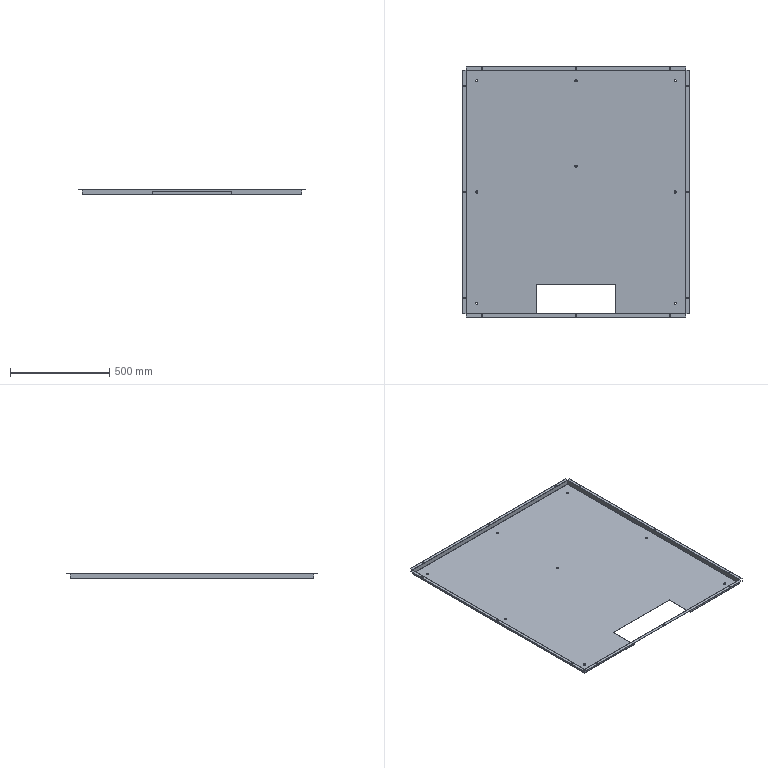Part | SolidWorks | features ICE 4, EdgeFlange 2, FlatPattern 1, SMBaseFlange 1, SheetMetal 1 | 1 solid | 150 faces | box 1140 x 1260 x 25 mm | volume 1476577 mm3 | plane 78 | cylinder 64 | spline 8 | commonest cylinder face diameters 7 x30 11 x16 0.4 x9 2.4 x9